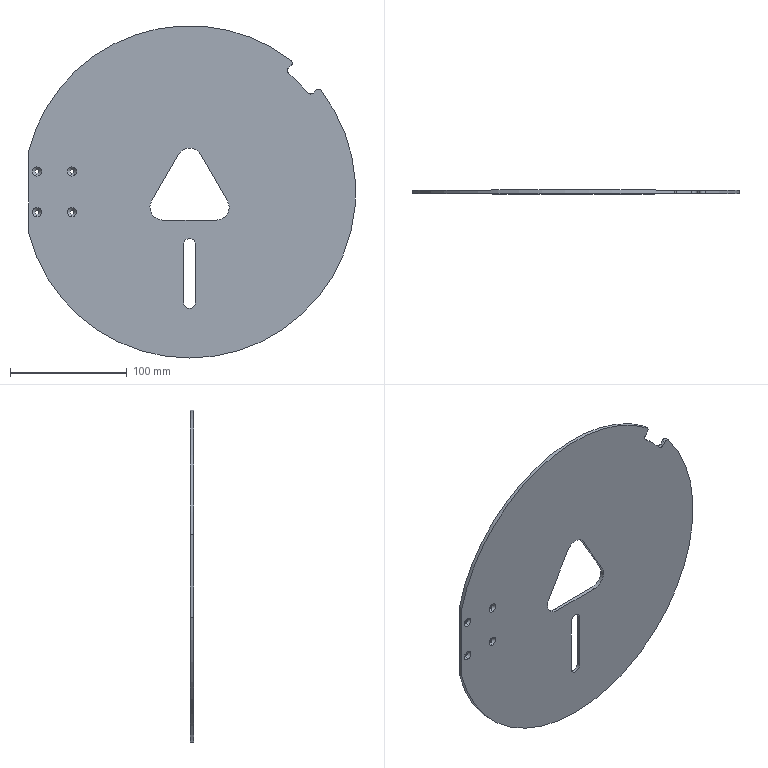Part | SolidWorks | features ICE 5, Chamfer 1, CirPattern 1, Cut 1, Extrusion 1, Fillet 1 | 1 solid | 41 faces | box 280.5 x 3 x 285 mm | volume 179414 mm3 | cylinder 23 | plane 10 | cone 8 | commonest cylinder face diameters 3.5 x8 6 x4 22 x4 10 x3 285 x3 265 x1
STEP:
#1=CARTESIAN_POINT('',(-100.892,2.2,-15.75));
#2=VERTEX_POINT('',#1);
#3=CARTESIAN_POINT('',(-100.892,2.2,-19.25));
#4=VERTEX_POINT('',#3);
#5=CARTESIAN_POINT('',(-100.892,2.2,-17.5));
#6=DIRECTION('',(0.,-1.,0.));
#7=DIRECTION('',(0.,0.,1.));
#8=AXIS2_PLACEMENT_3D('',#5,#6,#7);
#9=CIRCLE('',#8,1.75);
#10=EDGE_CURVE('',#2,#4,#9,.T.);
#11=ORIENTED_EDGE('',*,*,#10,.F.);
#12=CARTESIAN_POINT('',(-100.892,0.,-13.55));
#13=VERTEX_POINT('',#12);
#14=CARTESIAN_POINT('',(-100.892,0.,-13.55));
#15=DIRECTION('',(0.,-0.7071,0.7071));
#16=VECTOR('',#15,1000.);
#17=LINE('',#14,#16);
#18=EDGE_CURVE('',#2,#13,#17,.T.);
#19=ORIENTED_EDGE('',*,*,#18,.T.);
#20=CARTESIAN_POINT('',(-100.892,0.,-21.45));
#21=VERTEX_POINT('',#20);
#22=CARTESIAN_POINT('',(-100.892,0.,-17.5));
#23=DIRECTION('',(0.,1.,0.));
#24=DIRECTION('',(0.,0.,1.));
#25=AXIS2_PLACEMENT_3D('',#22,#23,#24);
#26=CIRCLE('',#25,3.95);
#27=EDGE_CURVE('',#21,#13,#26,.T.);
#28=ORIENTED_EDGE('',*,*,#27,.F.);
#29=CARTESIAN_POINT('',(-100.892,0.,-21.45));
#30=DIRECTION('',(0.,-0.7071,-0.7071));
#31=VECTOR('',#30,1000.);
#32=LINE('',#29,#31);
#33=EDGE_CURVE('',#4,#21,#32,.T.);
#34=ORIENTED_EDGE('',*,*,#33,.F.);
#35=EDGE_LOOP('',(#11,#19,#28,#34));
#36=FACE_OUTER_BOUND('',#35,.T.);
#37=CARTESIAN_POINT('',(-100.892,0.,-17.5));
#38=DIRECTION('',(0.,-1.,0.));
#39=DIRECTION('',(0.,0.,-1.));
#40=AXIS2_PLACEMENT_3D('',#37,#38,#39);
#41=CONICAL_SURFACE('',#40,3.95,0.7854);
#42=ADVANCED_FACE('',(#36),#41,.F.);
#43=CARTESIAN_POINT('',(-130.892,2.2,-15.75));
#44=VERTEX_POINT('',#43);
#45=CARTESIAN_POINT('',(-130.892,2.2,-19.25));
#46=VERTEX_POINT('',#45);
#47=CARTESIAN_POINT('',(-130.892,2.2,-17.5));
#48=DIRECTION('',(0.,-1.,0.));
#49=DIRECTION('',(0.,0.,1.));
#50=AXIS2_PLACEMENT_3D('',#47,#48,#49);
#51=CIRCLE('',#50,1.75);
#52=EDGE_CURVE('',#44,#46,#51,.T.);
#53=ORIENTED_EDGE('',*,*,#52,.F.);
#54=CARTESIAN_POINT('',(-130.892,0.,-13.55));
#55=VERTEX_POINT('',#54);
#56=CARTESIAN_POINT('',(-130.892,0.,-13.55));
#57=DIRECTION('',(0.,-0.7071,0.7071));
#58=VECTOR('',#57,1000.);
#59=LINE('',#56,#58);
#60=EDGE_CURVE('',#44,#55,#59,.T.);
#61=ORIENTED_EDGE('',*,*,#60,.T.);
#62=CARTESIAN_POINT('',(-130.892,0.,-21.45));
#63=VERTEX_POINT('',#62);
#64=CARTESIAN_POINT('',(-130.892,0.,-17.5));
#65=DIRECTION('',(0.,1.,0.));
#66=DIRECTION('',(0.,0.,1.));
#67=AXIS2_PLACEMENT_3D('',#64,#65,#66);
#68=CIRCLE('',#67,3.95);
#69=EDGE_CURVE('',#63,#55,#68,.T.);
#70=ORIENTED_EDGE('',*,*,#69,.F.);
#71=CARTESIAN_POINT('',(-130.892,0.,-21.45));
#72=DIRECTION('',(0.,-0.7071,-0.7071));
#73=VECTOR('',#72,1000.);
#74=LINE('',#71,#73);
#75=EDGE_CURVE('',#46,#63,#74,.T.);
#76=ORIENTED_EDGE('',*,*,#75,.F.);
#77=EDGE_LOOP('',(#53,#61,#70,#76));
#78=FACE_OUTER_BOUND('',#77,.T.);
#79=CARTESIAN_POINT('',(-130.892,0.,-17.5));
#80=DIRECTION('',(0.,-1.,0.));
#81=DIRECTION('',(0.,0.,-1.));
#82=AXIS2_PLACEMENT_3D('',#79,#80,#81);
#83=CONICAL_SURFACE('',#82,3.95,0.7854);
#84=ADVANCED_FACE('',(#78),#83,.F.);
#85=CARTESIAN_POINT('',(-100.892,2.2,19.25));
#86=VERTEX_POINT('',#85);
#87=CARTESIAN_POINT('',(-100.892,2.2,15.75));
#88=VERTEX_POINT('',#87);
#89=CARTESIAN_POINT('',(-100.892,2.2,17.5));
#90=DIRECTION('',(0.,-1.,0.));
#91=DIRECTION('',(0.,0.,1.));
#92=AXIS2_PLACEMENT_3D('',#89,#90,#91);
#93=CIRCLE('',#92,1.75);
#94=EDGE_CURVE('',#86,#88,#93,.T.);
#95=ORIENTED_EDGE('',*,*,#94,.F.);
#96=CARTESIAN_POINT('',(-100.892,0.,21.45));
#97=VERTEX_POINT('',#96);
#98=CARTESIAN_POINT('',(-100.892,0.,21.45));
#99=DIRECTION('',(0.,-0.7071,0.7071));
#100=VECTOR('',#99,1000.);
#101=LINE('',#98,#100);
#102=EDGE_CURVE('',#86,#97,#101,.T.);
#103=ORIENTED_EDGE('',*,*,#102,.T.);
#104=CARTESIAN_POINT('',(-100.892,0.,13.55));
#105=VERTEX_POINT('',#104);
#106=CARTESIAN_POINT('',(-100.892,0.,17.5));
#107=DIRECTION('',(0.,1.,0.));
#108=DIRECTION('',(0.,0.,1.));
#109=AXIS2_PLACEMENT_3D('',#106,#107,#108);
#110=CIRCLE('',#109,3.95);
#111=EDGE_CURVE('',#105,#97,#110,.T.);
#112=ORIENTED_EDGE('',*,*,#111,.F.);
#113=CARTESIAN_POINT('',(-100.892,0.,13.55));
#114=DIRECTION('',(0.,-0.7071,-0.7071));
#115=VECTOR('',#114,1000.);
#116=LINE('',#113,#115);
#117=EDGE_CURVE('',#88,#105,#116,.T.);
#118=ORIENTED_EDGE('',*,*,#117,.F.);
#119=EDGE_LOOP('',(#95,#103,#112,#118));
#120=FACE_OUTER_BOUND('',#119,.T.);
#121=CARTESIAN_POINT('',(-100.892,0.,17.5));
#122=DIRECTION('',(0.,-1.,0.));
#123=DIRECTION('',(0.,0.,-1.));
#124=AXIS2_PLACEMENT_3D('',#121,#122,#123);
#125=CONICAL_SURFACE('',#124,3.95,0.7854);
#126=ADVANCED_FACE('',(#120),#125,.F.);
#127=CARTESIAN_POINT('',(-130.892,2.2,19.25));
#128=VERTEX_POINT('',#127);
#129=CARTESIAN_POINT('',(-130.892,2.2,15.75));
#130=VERTEX_POINT('',#129);
#131=CARTESIAN_POINT('',(-130.892,2.2,17.5));
#132=DIRECTION('',(0.,-1.,0.));
#133=DIRECTION('',(0.,0.,1.));
#134=AXIS2_PLACEMENT_3D('',#131,#132,#133);
#135=CIRCLE('',#134,1.75);
#136=EDGE_CURVE('',#128,#130,#135,.T.);
#137=ORIENTED_EDGE('',*,*,#136,.F.);
#138=CARTESIAN_POINT('',(-130.892,0.,21.45));
#139=VERTEX_POINT('',#138);
#140=CARTESIAN_POINT('',(-130.892,0.,21.45));
#141=DIRECTION('',(0.,-0.7071,0.7071));
#142=VECTOR('',#141,1000.);
#143=LINE('',#140,#142);
#144=EDGE_CURVE('',#128,#139,#143,.T.);
#145=ORIENTED_EDGE('',*,*,#144,.T.);
#146=CARTESIAN_POINT('',(-130.892,0.,13.55));
#147=VERTEX_POINT('',#146);
#148=CARTESIAN_POINT('',(-130.892,0.,17.5));
#149=DIRECTION('',(0.,1.,0.));
#150=DIRECTION('',(0.,0.,1.));
#151=AXIS2_PLACEMENT_3D('',#148,#149,#150);
#152=CIRCLE('',#151,3.95);
#153=EDGE_CURVE('',#147,#139,#152,.T.);
#154=ORIENTED_EDGE('',*,*,#153,.F.);
#155=CARTESIAN_POINT('',(-130.892,0.,13.55));
#156=DIRECTION('',(0.,-0.7071,-0.7071));
#157=VECTOR('',#156,1000.);
#158=LINE('',#155,#157);
#159=EDGE_CURVE('',#130,#147,#158,.T.);
#160=ORIENTED_EDGE('',*,*,#159,.F.);
#161=EDGE_LOOP('',(#137,#145,#154,#160));
#162=FACE_OUTER_BOUND('',#161,.T.);
#163=CARTESIAN_POINT('',(-130.892,0.,17.5));
#164=DIRECTION('',(0.,-1.,0.));
#165=DIRECTION('',(0.,0.,-1.));
#166=AXIS2_PLACEMENT_3D('',#163,#164,#165);
#167=CONICAL_SURFACE('',#166,3.95,0.7854);
#168=ADVANCED_FACE('',(#162),#167,.F.);
#169=ORIENTED_EDGE('',*,*,#94,.T.);
#170=CARTESIAN_POINT('',(-100.892,3.,15.75));
#171=VERTEX_POINT('',#170);
#172=CARTESIAN_POINT('',(-100.892,-7.,15.75));
#173=DIRECTION('',(0.,1.,0.));
#174=VECTOR('',#173,1000.);
#175=LINE('',#172,#174);
#176=EDGE_CURVE('',#88,#171,#175,.T.);
#177=ORIENTED_EDGE('',*,*,#176,.T.);
#178=CARTESIAN_POINT('',(-100.892,3.,19.25));
#179=VERTEX_POINT('',#178);
#180=CARTESIAN_POINT('',(-100.892,3.,17.5));
#181=DIRECTION('',(0.,1.,0.));
#182=DIRECTION('',(0.,0.,1.));
#183=AXIS2_PLACEMENT_3D('',#180,#181,#182);
#184=CIRCLE('',#183,1.75);
#185=EDGE_CURVE('',#171,#179,#184,.T.);
#186=ORIENTED_EDGE('',*,*,#185,.T.);
#187=CARTESIAN_POINT('',(-100.892,-7.,19.25));
#188=DIRECTION('',(0.,1.,0.));
#189=VECTOR('',#188,1000.);
#190=LINE('',#187,#189);
#191=EDGE_CURVE('',#86,#179,#190,.T.);
#192=ORIENTED_EDGE('',*,*,#191,.F.);
#193=EDGE_LOOP('',(#169,#177,#186,#192));
#194=FACE_OUTER_BOUND('',#193,.T.);
#195=CARTESIAN_POINT('',(-100.892,-7.,17.5));
#196=DIRECTION('',(0.,1.,0.));
#197=DIRECTION('',(0.,0.,1.));
#198=AXIS2_PLACEMENT_3D('',#195,#196,#197);
#199=CYLINDRICAL_SURFACE('',#198,1.75);
#200=ADVANCED_FACE('',(#194),#199,.F.);
#201=ORIENTED_EDGE('',*,*,#136,.T.);
#202=CARTESIAN_POINT('',(-130.892,3.,15.75));
#203=VERTEX_POINT('',#202);
#204=CARTESIAN_POINT('',(-130.892,-7.,15.75));
#205=DIRECTION('',(0.,1.,0.));
#206=VECTOR('',#205,1000.);
#207=LINE('',#204,#206);
#208=EDGE_CURVE('',#130,#203,#207,.T.);
#209=ORIENTED_EDGE('',*,*,#208,.T.);
#210=CARTESIAN_POINT('',(-130.892,3.,19.25));
#211=VERTEX_POINT('',#210);
#212=CARTESIAN_POINT('',(-130.892,3.,17.5));
#213=DIRECTION('',(0.,1.,0.));
#214=DIRECTION('',(0.,0.,1.));
#215=AXIS2_PLACEMENT_3D('',#212,#213,#214);
#216=CIRCLE('',#215,1.75);
#217=EDGE_CURVE('',#203,#211,#216,.T.);
#218=ORIENTED_EDGE('',*,*,#217,.T.);
#219=CARTESIAN_POINT('',(-130.892,-7.,19.25));
#220=DIRECTION('',(0.,1.,0.));
#221=VECTOR('',#220,1000.);
#222=LINE('',#219,#221);
#223=EDGE_CURVE('',#128,#211,#222,.T.);
#224=ORIENTED_EDGE('',*,*,#223,.F.);
#225=EDGE_LOOP('',(#201,#209,#218,#224));
#226=FACE_OUTER_BOUND('',#225,.T.);
#227=CARTESIAN_POINT('',(-130.892,-7.,17.5));
#228=DIRECTION('',(0.,1.,0.));
#229=DIRECTION('',(0.,0.,1.));
#230=AXIS2_PLACEMENT_3D('',#227,#228,#229);
#231=CYLINDRICAL_SURFACE('',#230,1.75);
#232=ADVANCED_FACE('',(#226),#231,.F.);
#233=ORIENTED_EDGE('',*,*,#10,.T.);
#234=CARTESIAN_POINT('',(-100.892,3.,-19.25));
#235=VERTEX_POINT('',#234);
#236=CARTESIAN_POINT('',(-100.892,-7.,-19.25));
#237=DIRECTION('',(0.,1.,0.));
#238=VECTOR('',#237,1000.);
#239=LINE('',#236,#238);
#240=EDGE_CURVE('',#4,#235,#239,.T.);
#241=ORIENTED_EDGE('',*,*,#240,.T.);
#242=CARTESIAN_POINT('',(-100.892,3.,-15.75));
#243=VERTEX_POINT('',#242);
#244=CARTESIAN_POINT('',(-100.892,3.,-17.5));
#245=DIRECTION('',(0.,1.,0.));
#246=DIRECTION('',(0.,0.,1.));
#247=AXIS2_PLACEMENT_3D('',#244,#245,#246);
#248=CIRCLE('',#247,1.75);
#249=EDGE_CURVE('',#235,#243,#248,.T.);
#250=ORIENTED_EDGE('',*,*,#249,.T.);
#251=CARTESIAN_POINT('',(-100.892,-7.,-15.75));
#252=DIRECTION('',(0.,1.,0.));
#253=VECTOR('',#252,1000.);
#254=LINE('',#251,#253);
#255=EDGE_CURVE('',#2,#243,#254,.T.);
#256=ORIENTED_EDGE('',*,*,#255,.F.);
#257=EDGE_LOOP('',(#233,#241,#250,#256));
#258=FACE_OUTER_BOUND('',#257,.T.);
#259=CARTESIAN_POINT('',(-100.892,-7.,-17.5));
#260=DIRECTION('',(0.,1.,0.));
#261=DIRECTION('',(0.,0.,1.));
#262=AXIS2_PLACEMENT_3D('',#259,#260,#261);
#263=CYLINDRICAL_SURFACE('',#262,1.75);
#264=ADVANCED_FACE('',(#258),#263,.F.);
#265=ORIENTED_EDGE('',*,*,#52,.T.);
#266=CARTESIAN_POINT('',(-130.892,3.,-19.25));
#267=VERTEX_POINT('',#266);
#268=CARTESIAN_POINT('',(-130.892,-7.,-19.25));
#269=DIRECTION('',(0.,1.,0.));
#270=VECTOR('',#269,1000.);
#271=LINE('',#268,#270);
#272=EDGE_CURVE('',#46,#267,#271,.T.);
#273=ORIENTED_EDGE('',*,*,#272,.T.);
#274=CARTESIAN_POINT('',(-130.892,3.,-15.75));
#275=VERTEX_POINT('',#274);
#276=CARTESIAN_POINT('',(-130.892,3.,-17.5));
#277=DIRECTION('',(0.,1.,0.));
#278=DIRECTION('',(0.,0.,1.));
#279=AXIS2_PLACEMENT_3D('',#276,#277,#278);
#280=CIRCLE('',#279,1.75);
#281=EDGE_CURVE('',#267,#275,#280,.T.);
#282=ORIENTED_EDGE('',*,*,#281,.T.);
#283=CARTESIAN_POINT('',(-130.892,-7.,-15.75));
#284=DIRECTION('',(0.,1.,0.));
#285=VECTOR('',#284,1000.);
#286=LINE('',#283,#285);
#287=EDGE_CURVE('',#44,#275,#286,.T.);
#288=ORIENTED_EDGE('',*,*,#287,.F.);
#289=EDGE_LOOP('',(#265,#273,#282,#288));
#290=FACE_OUTER_BOUND('',#289,.T.);
#291=CARTESIAN_POINT('',(-130.892,-7.,-17.5));
#292=DIRECTION('',(0.,1.,0.));
#293=DIRECTION('',(0.,0.,1.));
#294=AXIS2_PLACEMENT_3D('',#291,#292,#293);
#295=CYLINDRICAL_SURFACE('',#294,1.75);
#296=ADVANCED_FACE('',(#290),#295,.F.);
#297=CARTESIAN_POINT('',(0.,0.,-40.));
#298=VERTEX_POINT('',#297);
#299=CARTESIAN_POINT('',(5.,0.,-45.));
#300=VERTEX_POINT('',#299);
#301=CARTESIAN_POINT('',(0.,0.,-45.));
#302=DIRECTION('',(0.,1.,0.));
#303=DIRECTION('',(0.,0.,1.));
#304=AXIS2_PLACEMENT_3D('',#301,#302,#303);
#305=CIRCLE('',#304,5.);
#306=EDGE_CURVE('',#298,#300,#305,.T.);
#307=ORIENTED_EDGE('',*,*,#306,.F.);
#308=CARTESIAN_POINT('',(0.,3.,-40.));
#309=VERTEX_POINT('',#308);
#310=CARTESIAN_POINT('',(0.,-7.,-40.));
#311=DIRECTION('',(0.,1.,0.));
#312=VECTOR('',#311,1000.);
#313=LINE('',#310,#312);
#314=EDGE_CURVE('',#298,#309,#313,.T.);
#315=ORIENTED_EDGE('',*,*,#314,.T.);
#316=CARTESIAN_POINT('',(5.,3.,-45.));
#317=VERTEX_POINT('',#316);
#318=CARTESIAN_POINT('',(0.,3.,-45.));
#319=DIRECTION('',(0.,1.,0.));
#320=DIRECTION('',(0.,0.,1.));
#321=AXIS2_PLACEMENT_3D('',#318,#319,#320);
#322=CIRCLE('',#321,5.);
#323=EDGE_CURVE('',#309,#317,#322,.T.);
#324=ORIENTED_EDGE('',*,*,#323,.T.);
#325=CARTESIAN_POINT('',(5.,-7.,-45.));
#326=DIRECTION('',(0.,1.,0.));
#327=VECTOR('',#326,1000.);
#328=LINE('',#325,#327);
#329=EDGE_CURVE('',#300,#317,#328,.T.);
#330=ORIENTED_EDGE('',*,*,#329,.F.);
#331=EDGE_LOOP('',(#307,#315,#324,#330));
#332=FACE_OUTER_BOUND('',#331,.T.);
#333=CARTESIAN_POINT('',(0.,-7.,-45.));
#334=DIRECTION('',(0.,1.,0.));
#335=DIRECTION('',(0.,0.,1.));
#336=AXIS2_PLACEMENT_3D('',#333,#334,#335);
#337=CYLINDRICAL_SURFACE('',#336,5.);
#338=ADVANCED_FACE('',(#332),#337,.F.);
#339=CARTESIAN_POINT('',(0.,3.,-142.5));
#340=VERTEX_POINT('',#339);
#341=CARTESIAN_POINT('',(-138.,3.,-35.528));
#342=VERTEX_POINT('',#341);
#343=CARTESIAN_POINT('',(0.,3.,0.));
#344=DIRECTION('',(0.,1.,0.));
#345=DIRECTION('',(0.,0.,1.));
#346=AXIS2_PLACEMENT_3D('',#343,#344,#345);
#347=CIRCLE('',#346,142.5);
#348=EDGE_CURVE('',#340,#342,#347,.T.);
#349=ORIENTED_EDGE('',*,*,#348,.F.);
#350=CARTESIAN_POINT('',(0.,0.,-142.5));
#351=VERTEX_POINT('',#350);
#352=CARTESIAN_POINT('',(0.,3.,-142.5));
#353=DIRECTION('',(0.,-1.,0.));
#354=VECTOR('',#353,1000.);
#355=LINE('',#352,#354);
#356=EDGE_CURVE('',#340,#351,#355,.T.);
#357=ORIENTED_EDGE('',*,*,#356,.T.);
#358=CARTESIAN_POINT('',(-138.,0.,-35.528));
#359=VERTEX_POINT('',#358);
#360=CARTESIAN_POINT('',(0.,0.,0.));
#361=DIRECTION('',(0.,1.,0.));
#362=DIRECTION('',(0.,0.,1.));
#363=AXIS2_PLACEMENT_3D('',#360,#361,#362);
#364=CIRCLE('',#363,142.5);
#365=EDGE_CURVE('',#351,#359,#364,.T.);
#366=ORIENTED_EDGE('',*,*,#365,.T.);
#367=CARTESIAN_POINT('',(-138.,3.,-35.528));
#368=DIRECTION('',(0.,1.,0.));
#369=VECTOR('',#368,1000.);
#370=LINE('',#367,#369);
#371=EDGE_CURVE('',#359,#342,#370,.T.);
#372=ORIENTED_EDGE('',*,*,#371,.T.);
#373=EDGE_LOOP('',(#349,#357,#366,#372));
#374=FACE_OUTER_BOUND('',#373,.T.);
#375=CARTESIAN_POINT('',(0.,3.,0.));
#376=DIRECTION('',(0.,-1.,0.));
#377=DIRECTION('',(0.,0.,-1.));
#378=AXIS2_PLACEMENT_3D('',#375,#376,#377);
#379=CYLINDRICAL_SURFACE('',#378,142.5);
#380=ADVANCED_FACE('',(#374),#379,.T.);
#381=CARTESIAN_POINT('',(0.,0.,37.5));
#382=VERTEX_POINT('',#381);
#383=CARTESIAN_POINT('',(9.526,0.,32.));
#384=VERTEX_POINT('',#383);
#385=CARTESIAN_POINT('',(0.,0.,26.5));
#386=DIRECTION('',(0.,1.,0.));
#387=DIRECTION('',(0.,0.,1.));
#388=AXIS2_PLACEMENT_3D('',#385,#386,#387);
#389=CIRCLE('',#388,11.);
#390=EDGE_CURVE('',#382,#384,#389,.T.);
#391=ORIENTED_EDGE('',*,*,#390,.F.);
#392=CARTESIAN_POINT('',(0.,3.,37.5));
#393=VERTEX_POINT('',#392);
#394=CARTESIAN_POINT('',(0.,-7.,37.5));
#395=DIRECTION('',(0.,1.,0.));
#396=VECTOR('',#395,1000.);
#397=LINE('',#394,#396);
#398=EDGE_CURVE('',#382,#393,#397,.T.);
#399=ORIENTED_EDGE('',*,*,#398,.T.);
#400=CARTESIAN_POINT('',(9.526,3.,32.));
#401=VERTEX_POINT('',#400);
#402=CARTESIAN_POINT('',(0.,3.,26.5));
#403=DIRECTION('',(0.,1.,0.));
#404=DIRECTION('',(0.,0.,1.));
#405=AXIS2_PLACEMENT_3D('',#402,#403,#404);
#406=CIRCLE('',#405,11.);
#407=EDGE_CURVE('',#393,#401,#406,.T.);
#408=ORIENTED_EDGE('',*,*,#407,.T.);
#409=CARTESIAN_POINT('',(9.526,-7.,32.));
#410=DIRECTION('',(0.,1.,0.));
#411=VECTOR('',#410,1000.);
#412=LINE('',#409,#411);
#413=EDGE_CURVE('',#384,#401,#412,.T.);
#414=ORIENTED_EDGE('',*,*,#413,.F.);
#415=EDGE_LOOP('',(#391,#399,#408,#414));
#416=FACE_OUTER_BOUND('',#415,.T.);
#417=CARTESIAN_POINT('',(0.,-7.,26.5));
#418=DIRECTION('',(0.,1.,0.));
#419=DIRECTION('',(0.,0.,1.));
#420=AXIS2_PLACEMENT_3D('',#417,#418,#419);
#421=CYLINDRICAL_SURFACE('',#420,11.);
#422=ADVANCED_FACE('',(#416),#421,.F.);
#423=CARTESIAN_POINT('',(-138.,3.,35.528));
#424=VERTEX_POINT('',#423);
#425=CARTESIAN_POINT('',(86.919,3.,112.922));
#426=VERTEX_POINT('',#425);
#427=CARTESIAN_POINT('',(0.,3.,0.));
#428=DIRECTION('',(0.,1.,0.));
#429=DIRECTION('',(0.,0.,1.));
#430=AXIS2_PLACEMENT_3D('',#427,#428,#429);
#431=CIRCLE('',#430,142.5);
#432=EDGE_CURVE('',#424,#426,#431,.T.);
#433=ORIENTED_EDGE('',*,*,#432,.F.);
#434=CARTESIAN_POINT('',(-138.,0.,35.528));
#435=VERTEX_POINT('',#434);
#436=CARTESIAN_POINT('',(-138.,3.,35.528));
#437=DIRECTION('',(0.,-1.,0.));
#438=VECTOR('',#437,1000.);
#439=LINE('',#436,#438);
#440=EDGE_CURVE('',#424,#435,#439,.T.);
#441=ORIENTED_EDGE('',*,*,#440,.T.);
#442=CARTESIAN_POINT('',(86.919,0.,112.922));
#443=VERTEX_POINT('',#442);
#444=CARTESIAN_POINT('',(0.,0.,0.));
#445=DIRECTION('',(0.,1.,0.));
#446=DIRECTION('',(0.,0.,1.));
#447=AXIS2_PLACEMENT_3D('',#444,#445,#446);
#448=CIRCLE('',#447,142.5);
#449=EDGE_CURVE('',#435,#443,#448,.T.);
#450=ORIENTED_EDGE('',*,*,#449,.T.);
#451=CARTESIAN_POINT('',(86.919,3.,112.922));
#452=DIRECTION('',(0.,1.,0.));
#453=VECTOR('',#452,1000.);
#454=LINE('',#451,#453);
#455=EDGE_CURVE('',#443,#426,#454,.T.);
#456=ORIENTED_EDGE('',*,*,#455,.T.);
#457=EDGE_LOOP('',(#433,#441,#450,#456));
#458=FACE_OUTER_BOUND('',#457,.T.);
#459=CARTESIAN_POINT('',(0.,3.,0.));
#460=DIRECTION('',(0.,-1.,0.));
#461=DIRECTION('',(0.,0.,-1.));
#462=AXIS2_PLACEMENT_3D('',#459,#460,#461);
#463=CYLINDRICAL_SURFACE('',#462,142.5);
#464=ADVANCED_FACE('',(#458),#463,.T.);
#465=ORIENTED_EDGE('',*,*,#398,.F.);
#466=CARTESIAN_POINT('',(-9.526,0.,32.));
#467=VERTEX_POINT('',#466);
#468=CARTESIAN_POINT('',(0.,0.,26.5));
#469=DIRECTION('',(0.,1.,0.));
#470=DIRECTION('',(0.,0.,1.));
#471=AXIS2_PLACEMENT_3D('',#468,#469,#470);
#472=CIRCLE('',#471,11.);
#473=EDGE_CURVE('',#467,#382,#472,.T.);
#474=ORIENTED_EDGE('',*,*,#473,.F.);
#475=CARTESIAN_POINT('',(-9.526,3.,32.));
#476=VERTEX_POINT('',#475);
#477=CARTESIAN_POINT('',(-9.526,-7.,32.));
#478=DIRECTION('',(0.,1.,0.));
#479=VECTOR('',#478,1000.);
#480=LINE('',#477,#479);
#481=EDGE_CURVE('',#467,#476,#480,.T.);
#482=ORIENTED_EDGE('',*,*,#481,.T.);
#483=CARTESIAN_POINT('',(0.,3.,26.5));
#484=DIRECTION('',(0.,1.,0.));
#485=DIRECTION('',(0.,0.,1.));
#486=AXIS2_PLACEMENT_3D('',#483,#484,#485);
#487=CIRCLE('',#486,11.);
#488=EDGE_CURVE('',#476,#393,#487,.T.);
#489=ORIENTED_EDGE('',*,*,#488,.T.);
#490=EDGE_LOOP('',(#465,#474,#482,#489));
#491=FACE_OUTER_BOUND('',#490,.T.);
#492=CARTESIAN_POINT('',(0.,-7.,26.5));
#493=DIRECTION('',(0.,1.,0.));
#494=DIRECTION('',(0.,0.,1.));
#495=AXIS2_PLACEMENT_3D('',#492,#493,#494);
#496=CYLINDRICAL_SURFACE('',#495,11.);
#497=ADVANCED_FACE('',(#491),#496,.F.);
#498=ORIENTED_EDGE('',*,*,#356,.F.);
#499=CARTESIAN_POINT('',(112.922,3.,86.919));
#500=VERTEX_POINT('',#499);
#501=CARTESIAN_POINT('',(0.,3.,0.));
#502=DIRECTION('',(0.,1.,0.));
#503=DIRECTION('',(0.,0.,1.));
#504=AXIS2_PLACEMENT_3D('',#501,#502,#503);
#505=CIRCLE('',#504,142.5);
#506=EDGE_CURVE('',#500,#340,#505,.T.);
#507=ORIENTED_EDGE('',*,*,#506,.F.);
#508=CARTESIAN_POINT('',(112.922,0.,86.919));
#509=VERTEX_POINT('',#508);
#510=CARTESIAN_POINT('',(112.922,3.,86.919));
#511=DIRECTION('',(0.,-1.,0.));
#512=VECTOR('',#511,1000.);
#513=LINE('',#510,#512);
#514=EDGE_CURVE('',#500,#509,#513,.T.);
#515=ORIENTED_EDGE('',*,*,#514,.T.);
#516=CARTESIAN_POINT('',(0.,0.,0.));
#517=DIRECTION('',(0.,1.,0.));
#518=DIRECTION('',(0.,0.,1.));
#519=AXIS2_PLACEMENT_3D('',#516,#517,#518);
#520=CIRCLE('',#519,142.5);
#521=EDGE_CURVE('',#509,#351,#520,.T.);
#522=ORIENTED_EDGE('',*,*,#521,.T.);
#523=EDGE_LOOP('',(#498,#507,#515,#522));
#524=FACE_OUTER_BOUND('',#523,.T.);
#525=CARTESIAN_POINT('',(0.,3.,0.));
#526=DIRECTION('',(0.,-1.,0.));
#527=DIRECTION('',(0.,0.,-1.));
#528=AXIS2_PLACEMENT_3D('',#525,#526,#527);
#529=CYLINDRICAL_SURFACE('',#528,142.5);
#530=ADVANCED_FACE('',(#524),#529,.T.);
#531=CARTESIAN_POINT('',(-100.892,3.,17.5));
#532=DIRECTION('',(0.,1.,0.));
#533=DIRECTION('',(0.,0.,1.));
#534=AXIS2_PLACEMENT_3D('',#531,#532,#533);
#535=CIRCLE('',#534,1.75);
#536=EDGE_CURVE('',#179,#171,#535,.T.);
#537=ORIENTED_EDGE('',*,*,#536,.F.);
#538=ORIENTED_EDGE('',*,*,#185,.F.);
#539=EDGE_LOOP('',(#537,#538));
#540=FACE_BOUND('',#539,.T.);
#541=CARTESIAN_POINT('',(-130.892,3.,17.5));
#542=DIRECTION('',(0.,1.,0.));
#543=DIRECTION('',(0.,0.,1.));
#544=AXIS2_PLACEMENT_3D('',#541,#542,#543);
#545=CIRCLE('',#544,1.75);
#546=EDGE_CURVE('',#211,#203,#545,.T.);
#547=ORIENTED_EDGE('',*,*,#546,.F.);
#548=ORIENTED_EDGE('',*,*,#217,.F.);
#549=EDGE_LOOP('',(#547,#548));
#550=FACE_BOUND('',#549,.T.);
#551=CARTESIAN_POINT('',(-100.892,3.,-17.5));
#552=DIRECTION('',(0.,1.,0.));
#553=DIRECTION('',(0.,0.,1.));
#554=AXIS2_PLACEMENT_3D('',#551,#552,#553);
#555=CIRCLE('',#554,1.75);
#556=EDGE_CURVE('',#243,#235,#555,.T.);
#557=ORIENTED_EDGE('',*,*,#556,.F.);
#558=ORIENTED_EDGE('',*,*,#249,.F.);
#559=EDGE_LOOP('',(#557,#558));
#560=FACE_BOUND('',#559,.T.);
#561=CARTESIAN_POINT('',(-130.892,3.,-17.5));
#562=DIRECTION('',(0.,1.,0.));
#563=DIRECTION('',(0.,0.,1.));
#564=AXIS2_PLACEMENT_3D('',#561,#562,#563);
#565=CIRCLE('',#564,1.75);
#566=EDGE_CURVE('',#275,#267,#565,.T.);
#567=ORIENTED_EDGE('',*,*,#566,.F.);
#568=ORIENTED_EDGE('',*,*,#281,.F.);
#569=EDGE_LOOP('',(#567,#568));
#570=FACE_BOUND('',#569,.T.);
#571=CARTESIAN_POINT('',(-138.,3.,-60.));
#572=DIRECTION('',(0.,0.,-1.));
#573=VECTOR('',#572,1000.);
#574=LINE('',#571,#573);
#575=EDGE_CURVE('',#424,#342,#574,.T.);
#576=ORIENTED_EDGE('',*,*,#575,.F.);
#577=ORIENTED_EDGE('',*,*,#432,.T.);
#578=CARTESIAN_POINT('',(87.21,3.,108.423));
#579=VERTEX_POINT('',#578);
#580=CARTESIAN_POINT('',(85.089,3.,110.545));
#581=DIRECTION('',(0.,1.,0.));
#582=DIRECTION('',(0.,0.,1.));
#583=AXIS2_PLACEMENT_3D('',#580,#581,#582);
#584=CIRCLE('',#583,3.);
#585=EDGE_CURVE('',#426,#579,#584,.T.);
#586=ORIENTED_EDGE('',*,*,#585,.T.);
#587=CARTESIAN_POINT('',(84.83,3.,106.043));
#588=VERTEX_POINT('',#587);
#589=CARTESIAN_POINT('',(89.596,3.,110.81));
#590=DIRECTION('',(0.7071,0.,0.7071));
#591=VECTOR('',#590,1000.);
#592=LINE('',#589,#591);
#593=EDGE_CURVE('',#588,#579,#592,.T.);
#594=ORIENTED_EDGE('',*,*,#593,.F.);
#595=CARTESIAN_POINT('',(85.026,3.,101.621));
#596=VERTEX_POINT('',#595);
#597=CARTESIAN_POINT('',(86.951,3.,103.922));
#598=DIRECTION('',(0.,-1.,0.));
#599=DIRECTION('',(0.,0.,1.));
#600=AXIS2_PLACEMENT_3D('',#597,#598,#599);
#601=CIRCLE('',#600,3.);
#602=EDGE_CURVE('',#588,#596,#601,.T.);
#603=ORIENTED_EDGE('',*,*,#602,.T.);
#604=CARTESIAN_POINT('',(101.621,3.,85.026));
#605=VERTEX_POINT('',#604);
#606=CARTESIAN_POINT('',(0.,3.,0.));
#607=DIRECTION('',(0.,-1.,0.));
#608=DIRECTION('',(0.,0.,1.));
#609=AXIS2_PLACEMENT_3D('',#606,#607,#608);
#610=CIRCLE('',#609,132.5);
#611=EDGE_CURVE('',#605,#596,#610,.T.);
#612=ORIENTED_EDGE('',*,*,#611,.F.);
#613=CARTESIAN_POINT('',(106.043,3.,84.83));
#614=VERTEX_POINT('',#613);
#615=CARTESIAN_POINT('',(103.922,3.,86.951));
#616=DIRECTION('',(0.,-1.,0.));
#617=DIRECTION('',(0.,0.,1.));
#618=AXIS2_PLACEMENT_3D('',#615,#616,#617);
#619=CIRCLE('',#618,3.);
#620=EDGE_CURVE('',#605,#614,#619,.T.);
#621=ORIENTED_EDGE('',*,*,#620,.T.);
#622=CARTESIAN_POINT('',(108.423,3.,87.21));
#623=VERTEX_POINT('',#622);
#624=CARTESIAN_POINT('',(110.81,3.,89.596));
#625=DIRECTION('',(-0.7071,0.,-0.7071));
#626=VECTOR('',#625,1000.);
#627=LINE('',#624,#626);
#628=EDGE_CURVE('',#623,#614,#627,.T.);
#629=ORIENTED_EDGE('',*,*,#628,.F.);
#630=CARTESIAN_POINT('',(110.545,3.,85.089));
#631=DIRECTION('',(0.,1.,0.));
#632=DIRECTION('',(0.,0.,1.));
#633=AXIS2_PLACEMENT_3D('',#630,#631,#632);
#634=CIRCLE('',#633,3.);
#635=EDGE_CURVE('',#623,#500,#634,.T.);
#636=ORIENTED_EDGE('',*,*,#635,.T.);
#637=ORIENTED_EDGE('',*,*,#506,.T.);
#638=ORIENTED_EDGE('',*,*,#348,.T.);
#639=EDGE_LOOP('',(#576,#577,#586,#594,#603,#612,#621,#629,#636,#637,#638));
#640=FACE_OUTER_BOUND('',#639,.T.);
#641=CARTESIAN_POINT('',(-5.,3.,-45.));
#642=VERTEX_POINT('',#641);
#643=CARTESIAN_POINT('',(0.,3.,-45.));
#644=DIRECTION('',(0.,1.,0.));
#645=DIRECTION('',(0.,0.,1.));
#646=AXIS2_PLACEMENT_3D('',#643,#644,#645);
#647=CIRCLE('',#646,5.);
#648=EDGE_CURVE('',#642,#309,#647,.T.);
#649=ORIENTED_EDGE('',*,*,#648,.F.);
#650=CARTESIAN_POINT('',(-5.,3.,-95.));
#651=VERTEX_POINT('',#650);
#652=CARTESIAN_POINT('',(-5.,3.,-45.));
#653=DIRECTION('',(0.,0.,1.));
#654=VECTOR('',#653,1000.);
#655=LINE('',#652,#654);
#656=EDGE_CURVE('',#651,#642,#655,.T.);
#657=ORIENTED_EDGE('',*,*,#656,.F.);
#658=CARTESIAN_POINT('',(5.,3.,-95.));
#659=VERTEX_POINT('',#658);
#660=CARTESIAN_POINT('',(0.,3.,-95.));
#661=DIRECTION('',(0.,1.,0.));
#662=DIRECTION('',(0.,0.,1.));
#663=AXIS2_PLACEMENT_3D('',#660,#661,#662);
#664=CIRCLE('',#663,5.);
#665=EDGE_CURVE('',#659,#651,#664,.T.);
#666=ORIENTED_EDGE('',*,*,#665,.F.);
#667=CARTESIAN_POINT('',(5.,3.,-45.));
#668=DIRECTION('',(0.,0.,-1.));
#669=VECTOR('',#668,1000.);
#670=LINE('',#667,#669);
#671=EDGE_CURVE('',#317,#659,#670,.T.);
#672=ORIENTED_EDGE('',*,*,#671,.F.);
#673=ORIENTED_EDGE('',*,*,#323,.F.);
#674=EDGE_LOOP('',(#649,#657,#666,#672,#673));
#675=FACE_BOUND('',#674,.T.);
#676=CARTESIAN_POINT('',(-32.476,3.,-7.75));
#677=VERTEX_POINT('',#676);
#678=CARTESIAN_POINT('',(-32.476,3.,-7.75));
#679=DIRECTION('',(0.5,0.,0.866));
#680=VECTOR('',#679,1000.);
#681=LINE('',#678,#680);
#682=EDGE_CURVE('',#677,#476,#681,.T.);
#683=ORIENTED_EDGE('',*,*,#682,.F.);
#684=CARTESIAN_POINT('',(-22.95,3.,-24.25));
#685=VERTEX_POINT('',#684);
#686=CARTESIAN_POINT('',(-22.95,3.,-13.25));
#687=DIRECTION('',(0.,1.,0.));
#688=DIRECTION('',(-0.866,0.,-0.5));
#689=AXIS2_PLACEMENT_3D('',#686,#687,#688);
#690=CIRCLE('',#689,11.);
#691=EDGE_CURVE('',#685,#677,#690,.T.);
#692=ORIENTED_EDGE('',*,*,#691,.F.);
#693=CARTESIAN_POINT('',(22.95,3.,-24.25));
#694=VERTEX_POINT('',#693);
#695=CARTESIAN_POINT('',(-22.95,3.,-24.25));
#696=DIRECTION('',(-1.,0.,0.));
#697=VECTOR('',#696,1000.);
#698=LINE('',#695,#697);
#699=EDGE_CURVE('',#694,#685,#698,.T.);
#700=ORIENTED_EDGE('',*,*,#699,.F.);
#701=CARTESIAN_POINT('',(32.476,3.,-7.75));
#702=VERTEX_POINT('',#701);
#703=CARTESIAN_POINT('',(22.95,3.,-13.25));
#704=DIRECTION('',(0.,1.,0.));
#705=DIRECTION('',(0.866,0.,-0.5));
#706=AXIS2_PLACEMENT_3D('',#703,#704,#705);
#707=CIRCLE('',#706,11.);
#708=EDGE_CURVE('',#702,#694,#707,.T.);
#709=ORIENTED_EDGE('',*,*,#708,.F.);
#710=CARTESIAN_POINT('',(32.476,3.,-7.75));
#711=DIRECTION('',(0.5,0.,-0.866));
#712=VECTOR('',#711,1000.);
#713=LINE('',#710,#712);
#714=EDGE_CURVE('',#401,#702,#713,.T.);
#715=ORIENTED_EDGE('',*,*,#714,.F.);
#716=ORIENTED_EDGE('',*,*,#407,.F.);
#717=ORIENTED_EDGE('',*,*,#488,.F.);
#718=EDGE_LOOP('',(#683,#692,#700,#709,#715,#716,#717));
#719=FACE_BOUND('',#718,.T.);
#720=CARTESIAN_POINT('',(0.,3.,0.));
#721=DIRECTION('',(0.,1.,0.));
#722=DIRECTION('',(0.,0.,1.));
#723=AXIS2_PLACEMENT_3D('',#720,#721,#722);
#724=PLANE('',#723);
#725=ADVANCED_FACE('',(#540,#550,#560,#570,#640,#675,#719),#724,.T.);
#726=ORIENTED_EDGE('',*,*,#153,.T.);
#727=CARTESIAN_POINT('',(-130.892,0.,17.5));
#728=DIRECTION('',(0.,1.,0.));
#729=DIRECTION('',(0.,0.,1.));
#730=AXIS2_PLACEMENT_3D('',#727,#728,#729);
#731=CIRCLE('',#730,3.95);
#732=EDGE_CURVE('',#139,#147,#731,.T.);
#733=ORIENTED_EDGE('',*,*,#732,.T.);
#734=EDGE_LOOP('',(#726,#733));
#735=FACE_BOUND('',#734,.T.);
#736=ORIENTED_EDGE('',*,*,#111,.T.);
#737=CARTESIAN_POINT('',(-100.892,0.,17.5));
#738=DIRECTION('',(0.,1.,0.));
#739=DIRECTION('',(0.,0.,1.));
#740=AXIS2_PLACEMENT_3D('',#737,#738,#739);
#741=CIRCLE('',#740,3.95);
#742=EDGE_CURVE('',#97,#105,#741,.T.);
#743=ORIENTED_EDGE('',*,*,#742,.T.);
#744=EDGE_LOOP('',(#736,#743));
#745=FACE_BOUND('',#744,.T.);
#746=ORIENTED_EDGE('',*,*,#69,.T.);
#747=CARTESIAN_POINT('',(-130.892,0.,-17.5));
#748=DIRECTION('',(0.,1.,0.));
#749=DIRECTION('',(0.,0.,1.));
#750=AXIS2_PLACEMENT_3D('',#747,#748,#749);
#751=CIRCLE('',#750,3.95);
#752=EDGE_CURVE('',#55,#63,#751,.T.);
#753=ORIENTED_EDGE('',*,*,#752,.T.);
#754=EDGE_LOOP('',(#746,#753));
#755=FACE_BOUND('',#754,.T.);
#756=ORIENTED_EDGE('',*,*,#27,.T.);
#757=CARTESIAN_POINT('',(-100.892,0.,-17.5));
#758=DIRECTION('',(0.,1.,0.));
#759=DIRECTION('',(0.,0.,1.));
#760=AXIS2_PLACEMENT_3D('',#757,#758,#759);
#761=CIRCLE('',#760,3.95);
#762=EDGE_CURVE('',#13,#21,#761,.T.);
#763=ORIENTED_EDGE('',*,*,#762,.T.);
#764=EDGE_LOOP('',(#756,#763));
#765=FACE_BOUND('',#764,.T.);
#766=CARTESIAN_POINT('',(-5.,0.,-95.));
#767=VERTEX_POINT('',#766);
#768=CARTESIAN_POINT('',(-5.,0.,-45.));
#769=VERTEX_POINT('',#768);
#770=CARTESIAN_POINT('',(-5.,0.,0.));
#771=DIRECTION('',(0.,0.,1.));
#772=VECTOR('',#771,1000.);
#773=LINE('',#770,#772);
#774=EDGE_CURVE('',#767,#769,#773,.T.);
#775=ORIENTED_EDGE('',*,*,#774,.T.);
#776=CARTESIAN_POINT('',(0.,0.,-45.));
#777=DIRECTION('',(0.,1.,0.));
#778=DIRECTION('',(0.,0.,1.));
#779=AXIS2_PLACEMENT_3D('',#776,#777,#778);
#780=CIRCLE('',#779,5.);
#781=EDGE_CURVE('',#769,#298,#780,.T.);
#782=ORIENTED_EDGE('',*,*,#781,.T.);
#783=ORIENTED_EDGE('',*,*,#306,.T.);
#784=CARTESIAN_POINT('',(5.,0.,-95.));
#785=VERTEX_POINT('',#784);
#786=CARTESIAN_POINT('',(5.,0.,0.));
#787=DIRECTION('',(0.,0.,-1.));
#788=VECTOR('',#787,1000.);
#789=LINE('',#786,#788);
#790=EDGE_CURVE('',#300,#785,#789,.T.);
#791=ORIENTED_EDGE('',*,*,#790,.T.);
#792=CARTESIAN_POINT('',(0.,0.,-95.));
#793=DIRECTION('',(0.,1.,0.));
#794=DIRECTION('',(0.,0.,1.));
#795=AXIS2_PLACEMENT_3D('',#792,#793,#794);
#796=CIRCLE('',#795,5.);
#797=EDGE_CURVE('',#785,#767,#796,.T.);
#798=ORIENTED_EDGE('',*,*,#797,.T.);
#799=EDGE_LOOP('',(#775,#782,#783,#791,#798));
#800=FACE_BOUND('',#799,.T.);
#801=CARTESIAN_POINT('',(-22.95,0.,-24.25));
#802=VERTEX_POINT('',#801);
#803=CARTESIAN_POINT('',(-32.476,0.,-7.75));
#804=VERTEX_POINT('',#803);
#805=CARTESIAN_POINT('',(-22.95,0.,-13.25));
#806=DIRECTION('',(0.,1.,0.));
#807=DIRECTION('',(0.,0.,1.));
#808=AXIS2_PLACEMENT_3D('',#805,#806,#807);
#809=CIRCLE('',#808,11.);
#810=EDGE_CURVE('',#802,#804,#809,.T.);
#811=ORIENTED_EDGE('',*,*,#810,.T.);
#812=CARTESIAN_POINT('',(-21.001,0.,12.125));
#813=DIRECTION('',(0.5,0.,0.866));
#814=VECTOR('',#813,1000.);
#815=LINE('',#812,#814);
#816=EDGE_CURVE('',#804,#467,#815,.T.);
#817=ORIENTED_EDGE('',*,*,#816,.T.);
#818=ORIENTED_EDGE('',*,*,#473,.T.);
#819=ORIENTED_EDGE('',*,*,#390,.T.);
#820=CARTESIAN_POINT('',(32.476,0.,-7.75));
#821=VERTEX_POINT('',#820);
#822=CARTESIAN_POINT('',(21.001,0.,12.125));
#823=DIRECTION('',(0.5,0.,-0.866));
#824=VECTOR('',#823,1000.);
#825=LINE('',#822,#824);
#826=EDGE_CURVE('',#384,#821,#825,.T.);
#827=ORIENTED_EDGE('',*,*,#826,.T.);
#828=CARTESIAN_POINT('',(22.95,0.,-24.25));
#829=VERTEX_POINT('',#828);
#830=CARTESIAN_POINT('',(22.95,0.,-13.25));
#831=DIRECTION('',(0.,1.,0.));
#832=DIRECTION('',(0.,0.,1.));
#833=AXIS2_PLACEMENT_3D('',#830,#831,#832);
#834=CIRCLE('',#833,11.);
#835=EDGE_CURVE('',#821,#829,#834,.T.);
#836=ORIENTED_EDGE('',*,*,#835,.T.);
#837=CARTESIAN_POINT('',(0.,0.,-24.25));
#838=DIRECTION('',(-1.,0.,0.));
#839=VECTOR('',#838,1000.);
#840=LINE('',#837,#839);
#841=EDGE_CURVE('',#829,#802,#840,.T.);
#842=ORIENTED_EDGE('',*,*,#841,.T.);
#843=EDGE_LOOP('',(#811,#817,#818,#819,#827,#836,#842));
#844=FACE_BOUND('',#843,.T.);
#845=ORIENTED_EDGE('',*,*,#449,.F.);
#846=CARTESIAN_POINT('',(-138.,0.,0.));
#847=DIRECTION('',(0.,0.,-1.));
#848=VECTOR('',#847,1000.);
#849=LINE('',#846,#848);
#850=EDGE_CURVE('',#435,#359,#849,.T.);
#851=ORIENTED_EDGE('',*,*,#850,.T.);
#852=ORIENTED_EDGE('',*,*,#365,.F.);
#853=ORIENTED_EDGE('',*,*,#521,.F.);
#854=CARTESIAN_POINT('',(108.423,0.,87.21));
#855=VERTEX_POINT('',#854);
#856=CARTESIAN_POINT('',(110.545,0.,85.089));
#857=DIRECTION('',(0.,-1.,0.));
#858=DIRECTION('',(0.,0.,1.));
#859=AXIS2_PLACEMENT_3D('',#856,#857,#858);
#860=CIRCLE('',#859,3.);
#861=EDGE_CURVE('',#509,#855,#860,.T.);
#862=ORIENTED_EDGE('',*,*,#861,.T.);
#863=CARTESIAN_POINT('',(106.043,0.,84.83));
#864=VERTEX_POINT('',#863);
#865=CARTESIAN_POINT('',(10.607,0.,-10.607));
#866=DIRECTION('',(-0.7071,0.,-0.7071));
#867=VECTOR('',#866,1000.);
#868=LINE('',#865,#867);
#869=EDGE_CURVE('',#855,#864,#868,.T.);
#870=ORIENTED_EDGE('',*,*,#869,.T.);
#871=CARTESIAN_POINT('',(101.621,0.,85.026));
#872=VERTEX_POINT('',#871);
#873=CARTESIAN_POINT('',(103.922,0.,86.951));
#874=DIRECTION('',(0.,1.,0.));
#875=DIRECTION('',(0.,0.,1.));
#876=AXIS2_PLACEMENT_3D('',#873,#874,#875);
#877=CIRCLE('',#876,3.);
#878=EDGE_CURVE('',#864,#872,#877,.T.);
#879=ORIENTED_EDGE('',*,*,#878,.T.);
#880=CARTESIAN_POINT('',(85.026,0.,101.621));
#881=VERTEX_POINT('',#880);
#882=CARTESIAN_POINT('',(0.,0.,0.));
#883=DIRECTION('',(0.,-1.,0.));
#884=DIRECTION('',(0.,0.,1.));
#885=AXIS2_PLACEMENT_3D('',#882,#883,#884);
#886=CIRCLE('',#885,132.5);
#887=EDGE_CURVE('',#872,#881,#886,.T.);
#888=ORIENTED_EDGE('',*,*,#887,.T.);
#889=CARTESIAN_POINT('',(84.83,0.,106.043));
#890=VERTEX_POINT('',#889);
#891=CARTESIAN_POINT('',(86.951,0.,103.922));
#892=DIRECTION('',(0.,1.,0.));
#893=DIRECTION('',(0.,0.,1.));
#894=AXIS2_PLACEMENT_3D('',#891,#892,#893);
#895=CIRCLE('',#894,3.);
#896=EDGE_CURVE('',#881,#890,#895,.T.);
#897=ORIENTED_EDGE('',*,*,#896,.T.);
#898=CARTESIAN_POINT('',(87.21,0.,108.423));
#899=VERTEX_POINT('',#898);
#900=CARTESIAN_POINT('',(-10.607,0.,10.607));
#901=DIRECTION('',(0.7071,0.,0.7071));
#902=VECTOR('',#901,1000.);
#903=LINE('',#900,#902);
#904=EDGE_CURVE('',#890,#899,#903,.T.);
#905=ORIENTED_EDGE('',*,*,#904,.T.);
#906=CARTESIAN_POINT('',(85.089,0.,110.545));
#907=DIRECTION('',(0.,-1.,0.));
#908=DIRECTION('',(0.,0.,1.));
#909=AXIS2_PLACEMENT_3D('',#906,#907,#908);
#910=CIRCLE('',#909,3.);
#911=EDGE_CURVE('',#899,#443,#910,.T.);
#912=ORIENTED_EDGE('',*,*,#911,.T.);
#913=EDGE_LOOP('',(#845,#851,#852,#853,#862,#870,#879,#888,#897,#905,#912));
#914=FACE_OUTER_BOUND('',#913,.T.);
#915=CARTESIAN_POINT('',(0.,0.,0.));
#916=DIRECTION('',(0.,1.,0.));
#917=DIRECTION('',(0.,0.,1.));
#918=AXIS2_PLACEMENT_3D('',#915,#916,#917);
#919=PLANE('',#918);
#920=ADVANCED_FACE('',(#735,#745,#755,#765,#800,#844,#914),#919,.F.);
#921=ORIENTED_EDGE('',*,*,#691,.T.);
#922=CARTESIAN_POINT('',(-32.476,-7.,-7.75));
#923=DIRECTION('',(0.,-1.,0.));
#924=VECTOR('',#923,1000.);
#925=LINE('',#922,#924);
#926=EDGE_CURVE('',#677,#804,#925,.T.);
#927=ORIENTED_EDGE('',*,*,#926,.T.);
#928=ORIENTED_EDGE('',*,*,#810,.F.);
#929=CARTESIAN_POINT('',(-22.95,-7.,-24.25));
#930=DIRECTION('',(0.,1.,0.));
#931=VECTOR('',#930,1000.);
#932=LINE('',#929,#931);
#933=EDGE_CURVE('',#802,#685,#932,.T.);
#934=ORIENTED_EDGE('',*,*,#933,.T.);
#935=EDGE_LOOP('',(#921,#927,#928,#934));
#936=FACE_OUTER_BOUND('',#935,.T.);
#937=CARTESIAN_POINT('',(-22.95,-7.,-13.25));
#938=DIRECTION('',(0.,1.,0.));
#939=DIRECTION('',(0.,0.,1.));
#940=AXIS2_PLACEMENT_3D('',#937,#938,#939);
#941=CYLINDRICAL_SURFACE('',#940,11.);
#942=ADVANCED_FACE('',(#936),#941,.F.);
#943=ORIENTED_EDGE('',*,*,#708,.T.);
#944=CARTESIAN_POINT('',(22.95,-7.,-24.25));
#945=DIRECTION('',(0.,-1.,0.));
#946=VECTOR('',#945,1000.);
#947=LINE('',#944,#946);
#948=EDGE_CURVE('',#694,#829,#947,.T.);
#949=ORIENTED_EDGE('',*,*,#948,.T.);
#950=ORIENTED_EDGE('',*,*,#835,.F.);
#951=CARTESIAN_POINT('',(32.476,-7.,-7.75));
#952=DIRECTION('',(0.,-1.,0.));
#953=VECTOR('',#952,1000.);
#954=LINE('',#951,#953);
#955=EDGE_CURVE('',#702,#821,#954,.T.);
#956=ORIENTED_EDGE('',*,*,#955,.F.);
#957=EDGE_LOOP('',(#943,#949,#950,#956));
#958=FACE_OUTER_BOUND('',#957,.T.);
#959=CARTESIAN_POINT('',(22.95,-7.,-13.25));
#960=DIRECTION('',(0.,1.,0.));
#961=DIRECTION('',(0.,0.,1.));
#962=AXIS2_PLACEMENT_3D('',#959,#960,#961);
#963=CYLINDRICAL_SURFACE('',#962,11.);
#964=ADVANCED_FACE('',(#958),#963,.F.);
#965=ORIENTED_EDGE('',*,*,#413,.T.);
#966=ORIENTED_EDGE('',*,*,#714,.T.);
#967=ORIENTED_EDGE('',*,*,#955,.T.);
#968=ORIENTED_EDGE('',*,*,#826,.F.);
#969=EDGE_LOOP('',(#965,#966,#967,#968));
#970=FACE_OUTER_BOUND('',#969,.T.);
#971=CARTESIAN_POINT('',(32.476,-7.,-7.75));
#972=DIRECTION('',(0.866,0.,0.5));
#973=DIRECTION('',(0.5,0.,-0.866));
#974=AXIS2_PLACEMENT_3D('',#971,#972,#973);
#975=PLANE('',#974);
#976=ADVANCED_FACE('',(#970),#975,.F.);
#977=ORIENTED_EDGE('',*,*,#948,.F.);
#978=ORIENTED_EDGE('',*,*,#699,.T.);
#979=ORIENTED_EDGE('',*,*,#933,.F.);
#980=ORIENTED_EDGE('',*,*,#841,.F.);
#981=EDGE_LOOP('',(#977,#978,#979,#980));
#982=FACE_OUTER_BOUND('',#981,.T.);
#983=CARTESIAN_POINT('',(-22.95,-7.,-24.25));
#984=DIRECTION('',(0.,0.,-1.));
#985=DIRECTION('',(-1.,0.,0.));
#986=AXIS2_PLACEMENT_3D('',#983,#984,#985);
#987=PLANE('',#986);
#988=ADVANCED_FACE('',(#982),#987,.F.);
#989=ORIENTED_EDGE('',*,*,#926,.F.);
#990=ORIENTED_EDGE('',*,*,#682,.T.);
#991=ORIENTED_EDGE('',*,*,#481,.F.);
#992=ORIENTED_EDGE('',*,*,#816,.F.);
#993=EDGE_LOOP('',(#989,#990,#991,#992));
#994=FACE_OUTER_BOUND('',#993,.T.);
#995=CARTESIAN_POINT('',(-32.476,-7.,-7.75));
#996=DIRECTION('',(-0.866,0.,0.5));
#997=DIRECTION('',(0.5,0.,0.866));
#998=AXIS2_PLACEMENT_3D('',#995,#996,#997);
#999=PLANE('',#998);
#1000=ADVANCED_FACE('',(#994),#999,.F.);
#1001=ORIENTED_EDGE('',*,*,#314,.F.);
#1002=ORIENTED_EDGE('',*,*,#781,.F.);
#1003=CARTESIAN_POINT('',(-5.,-7.,-45.));
#1004=DIRECTION('',(0.,1.,0.));
#1005=VECTOR('',#1004,1000.);
#1006=LINE('',#1003,#1005);
#1007=EDGE_CURVE('',#769,#642,#1006,.T.);
#1008=ORIENTED_EDGE('',*,*,#1007,.T.);
#1009=ORIENTED_EDGE('',*,*,#648,.T.);
#1010=EDGE_LOOP('',(#1001,#1002,#1008,#1009));
#1011=FACE_OUTER_BOUND('',#1010,.T.);
#1012=CARTESIAN_POINT('',(0.,-7.,-45.));
#1013=DIRECTION('',(0.,1.,0.));
#1014=DIRECTION('',(0.,0.,1.));
#1015=AXIS2_PLACEMENT_3D('',#1012,#1013,#1014);
#1016=CYLINDRICAL_SURFACE('',#1015,5.);
#1017=ADVANCED_FACE('',(#1011),#1016,.F.);
#1018=CARTESIAN_POINT('',(-5.,-7.,-95.));
#1019=DIRECTION('',(0.,1.,0.));
#1020=VECTOR('',#1019,1000.);
#1021=LINE('',#1018,#1020);
#1022=EDGE_CURVE('',#767,#651,#1021,.T.);
#1023=ORIENTED_EDGE('',*,*,#1022,.T.);
#1024=ORIENTED_EDGE('',*,*,#656,.T.);
#1025=ORIENTED_EDGE('',*,*,#1007,.F.);
#1026=ORIENTED_EDGE('',*,*,#774,.F.);
#1027=EDGE_LOOP('',(#1023,#1024,#1025,#1026));
#1028=FACE_OUTER_BOUND('',#1027,.T.);
#1029=CARTESIAN_POINT('',(-5.,-7.,-45.));
#1030=DIRECTION('',(-1.,0.,0.));
#1031=DIRECTION('',(0.,0.,1.));
#1032=AXIS2_PLACEMENT_3D('',#1029,#1030,#1031);
#1033=PLANE('',#1032);
#1034=ADVANCED_FACE('',(#1028),#1033,.F.);
#1035=CARTESIAN_POINT('',(5.,-7.,-95.));
#1036=DIRECTION('',(0.,1.,0.));
#1037=VECTOR('',#1036,1000.);
#1038=LINE('',#1035,#1037);
#1039=EDGE_CURVE('',#785,#659,#1038,.T.);
#1040=ORIENTED_EDGE('',*,*,#1039,.T.);
#1041=ORIENTED_EDGE('',*,*,#665,.T.);
#1042=ORIENTED_EDGE('',*,*,#1022,.F.);
#1043=ORIENTED_EDGE('',*,*,#797,.F.);
#1044=EDGE_LOOP('',(#1040,#1041,#1042,#1043));
#1045=FACE_OUTER_BOUND('',#1044,.T.);
#1046=CARTESIAN_POINT('',(0.,-7.,-95.));
#1047=DIRECTION('',(0.,1.,0.));
#1048=DIRECTION('',(0.,0.,1.));
#1049=AXIS2_PLACEMENT_3D('',#1046,#1047,#1048);
#1050=CYLINDRICAL_SURFACE('',#1049,5.);
#1051=ADVANCED_FACE('',(#1045),#1050,.F.);
#1052=ORIENTED_EDGE('',*,*,#329,.T.);
#1053=ORIENTED_EDGE('',*,*,#671,.T.);
#1054=ORIENTED_EDGE('',*,*,#1039,.F.);
#1055=ORIENTED_EDGE('',*,*,#790,.F.);
#1056=EDGE_LOOP('',(#1052,#1053,#1054,#1055));
#1057=FACE_OUTER_BOUND('',#1056,.T.);
#1058=CARTESIAN_POINT('',(5.,-7.,-45.));
#1059=DIRECTION('',(1.,0.,0.));
#1060=DIRECTION('',(0.,0.,-1.));
#1061=AXIS2_PLACEMENT_3D('',#1058,#1059,#1060);
#1062=PLANE('',#1061);
#1063=ADVANCED_FACE('',(#1057),#1062,.F.);
#1064=ORIENTED_EDGE('',*,*,#887,.F.);
#1065=CARTESIAN_POINT('',(101.621,-7.,85.026));
#1066=DIRECTION('',(0.,1.,0.));
#1067=VECTOR('',#1066,1000.);
#1068=LINE('',#1065,#1067);
#1069=EDGE_CURVE('',#872,#605,#1068,.T.);
#1070=ORIENTED_EDGE('',*,*,#1069,.T.);
#1071=ORIENTED_EDGE('',*,*,#611,.T.);
#1072=CARTESIAN_POINT('',(85.026,-7.,101.621));
#1073=DIRECTION('',(0.,-1.,0.));
#1074=VECTOR('',#1073,1000.);
#1075=LINE('',#1072,#1074);
#1076=EDGE_CURVE('',#596,#881,#1075,.T.);
#1077=ORIENTED_EDGE('',*,*,#1076,.T.);
#1078=EDGE_LOOP('',(#1064,#1070,#1071,#1077));
#1079=FACE_OUTER_BOUND('',#1078,.T.);
#1080=CARTESIAN_POINT('',(0.,-7.,0.));
#1081=DIRECTION('',(0.,1.,0.));
#1082=DIRECTION('',(0.,0.,1.));
#1083=AXIS2_PLACEMENT_3D('',#1080,#1081,#1082);
#1084=CYLINDRICAL_SURFACE('',#1083,132.5);
#1085=ADVANCED_FACE('',(#1079),#1084,.T.);
#1086=ORIENTED_EDGE('',*,*,#869,.F.);
#1087=CARTESIAN_POINT('',(108.423,-7.,87.21));
#1088=DIRECTION('',(0.,1.,0.));
#1089=VECTOR('',#1088,1000.);
#1090=LINE('',#1087,#1089);
#1091=EDGE_CURVE('',#855,#623,#1090,.T.);
#1092=ORIENTED_EDGE('',*,*,#1091,.T.);
#1093=ORIENTED_EDGE('',*,*,#628,.T.);
#1094=CARTESIAN_POINT('',(106.043,0.,84.83));
#1095=DIRECTION('',(0.,-1.,0.));
#1096=VECTOR('',#1095,1000.);
#1097=LINE('',#1094,#1096);
#1098=EDGE_CURVE('',#614,#864,#1097,.T.);
#1099=ORIENTED_EDGE('',*,*,#1098,.T.);
#1100=EDGE_LOOP('',(#1086,#1092,#1093,#1099));
#1101=FACE_OUTER_BOUND('',#1100,.T.);
#1102=CARTESIAN_POINT('',(110.81,-7.,89.596));
#1103=DIRECTION('',(0.7071,0.,-0.7071));
#1104=DIRECTION('',(-0.7071,0.,-0.7071));
#1105=AXIS2_PLACEMENT_3D('',#1102,#1103,#1104);
#1106=PLANE('',#1105);
#1107=ADVANCED_FACE('',(#1101),#1106,.F.);
#1108=ORIENTED_EDGE('',*,*,#593,.T.);
#1109=CARTESIAN_POINT('',(87.21,-7.,108.423));
#1110=DIRECTION('',(0.,-1.,0.));
#1111=VECTOR('',#1110,1000.);
#1112=LINE('',#1109,#1111);
#1113=EDGE_CURVE('',#579,#899,#1112,.T.);
#1114=ORIENTED_EDGE('',*,*,#1113,.T.);
#1115=ORIENTED_EDGE('',*,*,#904,.F.);
#1116=CARTESIAN_POINT('',(84.83,3.,106.043));
#1117=DIRECTION('',(0.,1.,0.));
#1118=VECTOR('',#1117,1000.);
#1119=LINE('',#1116,#1118);
#1120=EDGE_CURVE('',#890,#588,#1119,.T.);
#1121=ORIENTED_EDGE('',*,*,#1120,.T.);
#1122=EDGE_LOOP('',(#1108,#1114,#1115,#1121));
#1123=FACE_OUTER_BOUND('',#1122,.T.);
#1124=CARTESIAN_POINT('',(89.596,-7.,110.81));
#1125=DIRECTION('',(-0.7071,0.,0.7071));
#1126=DIRECTION('',(0.7071,0.,0.7071));
#1127=AXIS2_PLACEMENT_3D('',#1124,#1125,#1126);
#1128=PLANE('',#1127);
#1129=ADVANCED_FACE('',(#1123),#1128,.F.);
#1130=ORIENTED_EDGE('',*,*,#911,.F.);
#1131=ORIENTED_EDGE('',*,*,#1113,.F.);
#1132=ORIENTED_EDGE('',*,*,#585,.F.);
#1133=ORIENTED_EDGE('',*,*,#455,.F.);
#1134=EDGE_LOOP('',(#1130,#1131,#1132,#1133));
#1135=FACE_OUTER_BOUND('',#1134,.T.);
#1136=CARTESIAN_POINT('',(85.089,3.,110.545));
#1137=DIRECTION('',(0.,-1.,0.));
#1138=DIRECTION('',(0.,0.,-1.));
#1139=AXIS2_PLACEMENT_3D('',#1136,#1137,#1138);
#1140=CYLINDRICAL_SURFACE('',#1139,3.);
#1141=ADVANCED_FACE('',(#1135),#1140,.T.);
#1142=ORIENTED_EDGE('',*,*,#861,.F.);
#1143=ORIENTED_EDGE('',*,*,#514,.F.);
#1144=ORIENTED_EDGE('',*,*,#635,.F.);
#1145=ORIENTED_EDGE('',*,*,#1091,.F.);
#1146=EDGE_LOOP('',(#1142,#1143,#1144,#1145));
#1147=FACE_OUTER_BOUND('',#1146,.T.);
#1148=CARTESIAN_POINT('',(110.545,3.,85.089));
#1149=DIRECTION('',(0.,-1.,0.));
#1150=DIRECTION('',(0.,0.,-1.));
#1151=AXIS2_PLACEMENT_3D('',#1148,#1149,#1150);
#1152=CYLINDRICAL_SURFACE('',#1151,3.);
#1153=ADVANCED_FACE('',(#1147),#1152,.T.);
#1154=ORIENTED_EDGE('',*,*,#878,.F.);
#1155=ORIENTED_EDGE('',*,*,#1098,.F.);
#1156=ORIENTED_EDGE('',*,*,#620,.F.);
#1157=ORIENTED_EDGE('',*,*,#1069,.F.);
#1158=EDGE_LOOP('',(#1154,#1155,#1156,#1157));
#1159=FACE_OUTER_BOUND('',#1158,.T.);
#1160=CARTESIAN_POINT('',(103.922,-7.,86.951));
#1161=DIRECTION('',(0.,1.,0.));
#1162=DIRECTION('',(0.,0.,1.));
#1163=AXIS2_PLACEMENT_3D('',#1160,#1161,#1162);
#1164=CYLINDRICAL_SURFACE('',#1163,3.);
#1165=ADVANCED_FACE('',(#1159),#1164,.F.);
#1166=ORIENTED_EDGE('',*,*,#896,.F.);
#1167=ORIENTED_EDGE('',*,*,#1076,.F.);
#1168=ORIENTED_EDGE('',*,*,#602,.F.);
#1169=ORIENTED_EDGE('',*,*,#1120,.F.);
#1170=EDGE_LOOP('',(#1166,#1167,#1168,#1169));
#1171=FACE_OUTER_BOUND('',#1170,.T.);
#1172=CARTESIAN_POINT('',(86.951,-7.,103.922));
#1173=DIRECTION('',(0.,1.,0.));
#1174=DIRECTION('',(0.,0.,1.));
#1175=AXIS2_PLACEMENT_3D('',#1172,#1173,#1174);
#1176=CYLINDRICAL_SURFACE('',#1175,3.);
#1177=ADVANCED_FACE('',(#1171),#1176,.F.);
#1178=ORIENTED_EDGE('',*,*,#575,.T.);
#1179=ORIENTED_EDGE('',*,*,#371,.F.);
#1180=ORIENTED_EDGE('',*,*,#850,.F.);
#1181=ORIENTED_EDGE('',*,*,#440,.F.);
#1182=EDGE_LOOP('',(#1178,#1179,#1180,#1181));
#1183=FACE_OUTER_BOUND('',#1182,.T.);
#1184=CARTESIAN_POINT('',(-138.,-7.,-60.));
#1185=DIRECTION('',(1.,0.,0.));
#1186=DIRECTION('',(0.,0.,-1.));
#1187=AXIS2_PLACEMENT_3D('',#1184,#1185,#1186);
#1188=PLANE('',#1187);
#1189=ADVANCED_FACE('',(#1183),#1188,.F.);
#1190=ORIENTED_EDGE('',*,*,#272,.F.);
#1191=CARTESIAN_POINT('',(-130.892,2.2,-17.5));
#1192=DIRECTION('',(0.,-1.,0.));
#1193=DIRECTION('',(0.,0.,1.));
#1194=AXIS2_PLACEMENT_3D('',#1191,#1192,#1193);
#1195=CIRCLE('',#1194,1.75);
#1196=EDGE_CURVE('',#46,#44,#1195,.T.);
#1197=ORIENTED_EDGE('',*,*,#1196,.T.);
#1198=ORIENTED_EDGE('',*,*,#287,.T.);
#1199=ORIENTED_EDGE('',*,*,#566,.T.);
#1200=EDGE_LOOP('',(#1190,#1197,#1198,#1199));
#1201=FACE_OUTER_BOUND('',#1200,.T.);
#1202=CARTESIAN_POINT('',(-130.892,-7.,-17.5));
#1203=DIRECTION('',(0.,1.,0.));
#1204=DIRECTION('',(0.,0.,1.));
#1205=AXIS2_PLACEMENT_3D('',#1202,#1203,#1204);
#1206=CYLINDRICAL_SURFACE('',#1205,1.75);
#1207=ADVANCED_FACE('',(#1201),#1206,.F.);
#1208=ORIENTED_EDGE('',*,*,#240,.F.);
#1209=CARTESIAN_POINT('',(-100.892,2.2,-17.5));
#1210=DIRECTION('',(0.,-1.,0.));
#1211=DIRECTION('',(0.,0.,1.));
#1212=AXIS2_PLACEMENT_3D('',#1209,#1210,#1211);
#1213=CIRCLE('',#1212,1.75);
#1214=EDGE_CURVE('',#4,#2,#1213,.T.);
#1215=ORIENTED_EDGE('',*,*,#1214,.T.);
#1216=ORIENTED_EDGE('',*,*,#255,.T.);
#1217=ORIENTED_EDGE('',*,*,#556,.T.);
#1218=EDGE_LOOP('',(#1208,#1215,#1216,#1217));
#1219=FACE_OUTER_BOUND('',#1218,.T.);
#1220=CARTESIAN_POINT('',(-100.892,-7.,-17.5));
#1221=DIRECTION('',(0.,1.,0.));
#1222=DIRECTION('',(0.,0.,1.));
#1223=AXIS2_PLACEMENT_3D('',#1220,#1221,#1222);
#1224=CYLINDRICAL_SURFACE('',#1223,1.75);
#1225=ADVANCED_FACE('',(#1219),#1224,.F.);
#1226=ORIENTED_EDGE('',*,*,#208,.F.);
#1227=CARTESIAN_POINT('',(-130.892,2.2,17.5));
#1228=DIRECTION('',(0.,-1.,0.));
#1229=DIRECTION('',(0.,0.,1.));
#1230=AXIS2_PLACEMENT_3D('',#1227,#1228,#1229);
#1231=CIRCLE('',#1230,1.75);
#1232=EDGE_CURVE('',#130,#128,#1231,.T.);
#1233=ORIENTED_EDGE('',*,*,#1232,.T.);
#1234=ORIENTED_EDGE('',*,*,#223,.T.);
#1235=ORIENTED_EDGE('',*,*,#546,.T.);
#1236=EDGE_LOOP('',(#1226,#1233,#1234,#1235));
#1237=FACE_OUTER_BOUND('',#1236,.T.);
#1238=CARTESIAN_POINT('',(-130.892,-7.,17.5));
#1239=DIRECTION('',(0.,1.,0.));
#1240=DIRECTION('',(0.,0.,1.));
#1241=AXIS2_PLACEMENT_3D('',#1238,#1239,#1240);
#1242=CYLINDRICAL_SURFACE('',#1241,1.75);
#1243=ADVANCED_FACE('',(#1237),#1242,.F.);
#1244=ORIENTED_EDGE('',*,*,#176,.F.);
#1245=CARTESIAN_POINT('',(-100.892,2.2,17.5));
#1246=DIRECTION('',(0.,-1.,0.));
#1247=DIRECTION('',(0.,0.,1.));
#1248=AXIS2_PLACEMENT_3D('',#1245,#1246,#1247);
#1249=CIRCLE('',#1248,1.75);
#1250=EDGE_CURVE('',#88,#86,#1249,.T.);
#1251=ORIENTED_EDGE('',*,*,#1250,.T.);
#1252=ORIENTED_EDGE('',*,*,#191,.T.);
#1253=ORIENTED_EDGE('',*,*,#536,.T.);
#1254=EDGE_LOOP('',(#1244,#1251,#1252,#1253));
#1255=FACE_OUTER_BOUND('',#1254,.T.);
#1256=CARTESIAN_POINT('',(-100.892,-7.,17.5));
#1257=DIRECTION('',(0.,1.,0.));
#1258=DIRECTION('',(0.,0.,1.));
#1259=AXIS2_PLACEMENT_3D('',#1256,#1257,#1258);
#1260=CYLINDRICAL_SURFACE('',#1259,1.75);
#1261=ADVANCED_FACE('',(#1255),#1260,.F.);
#1262=ORIENTED_EDGE('',*,*,#144,.F.);
#1263=ORIENTED_EDGE('',*,*,#1232,.F.);
#1264=ORIENTED_EDGE('',*,*,#159,.T.);
#1265=ORIENTED_EDGE('',*,*,#732,.F.);
#1266=EDGE_LOOP('',(#1262,#1263,#1264,#1265));
#1267=FACE_OUTER_BOUND('',#1266,.T.);
#1268=CARTESIAN_POINT('',(-130.892,0.,17.5));
#1269=DIRECTION('',(0.,-1.,0.));
#1270=DIRECTION('',(0.,0.,-1.));
#1271=AXIS2_PLACEMENT_3D('',#1268,#1269,#1270);
#1272=CONICAL_SURFACE('',#1271,3.95,0.7854);
#1273=ADVANCED_FACE('',(#1267),#1272,.F.);
#1274=ORIENTED_EDGE('',*,*,#102,.F.);
#1275=ORIENTED_EDGE('',*,*,#1250,.F.);
#1276=ORIENTED_EDGE('',*,*,#117,.T.);
#1277=ORIENTED_EDGE('',*,*,#742,.F.);
#1278=EDGE_LOOP('',(#1274,#1275,#1276,#1277));
#1279=FACE_OUTER_BOUND('',#1278,.T.);
#1280=CARTESIAN_POINT('',(-100.892,0.,17.5));
#1281=DIRECTION('',(0.,-1.,0.));
#1282=DIRECTION('',(0.,0.,-1.));
#1283=AXIS2_PLACEMENT_3D('',#1280,#1281,#1282);
#1284=CONICAL_SURFACE('',#1283,3.95,0.7854);
#1285=ADVANCED_FACE('',(#1279),#1284,.F.);
#1286=ORIENTED_EDGE('',*,*,#60,.F.);
#1287=ORIENTED_EDGE('',*,*,#1196,.F.);
#1288=ORIENTED_EDGE('',*,*,#75,.T.);
#1289=ORIENTED_EDGE('',*,*,#752,.F.);
#1290=EDGE_LOOP('',(#1286,#1287,#1288,#1289));
#1291=FACE_OUTER_BOUND('',#1290,.T.);
#1292=CARTESIAN_POINT('',(-130.892,0.,-17.5));
#1293=DIRECTION('',(0.,-1.,0.));
#1294=DIRECTION('',(0.,0.,-1.));
#1295=AXIS2_PLACEMENT_3D('',#1292,#1293,#1294);
#1296=CONICAL_SURFACE('',#1295,3.95,0.7854);
#1297=ADVANCED_FACE('',(#1291),#1296,.F.);
#1298=ORIENTED_EDGE('',*,*,#18,.F.);
#1299=ORIENTED_EDGE('',*,*,#1214,.F.);
#1300=ORIENTED_EDGE('',*,*,#33,.T.);
#1301=ORIENTED_EDGE('',*,*,#762,.F.);
#1302=EDGE_LOOP('',(#1298,#1299,#1300,#1301));
#1303=FACE_OUTER_BOUND('',#1302,.T.);
#1304=CARTESIAN_POINT('',(-100.892,0.,-17.5));
#1305=DIRECTION('',(0.,-1.,0.));
#1306=DIRECTION('',(0.,0.,-1.));
#1307=AXIS2_PLACEMENT_3D('',#1304,#1305,#1306);
#1308=CONICAL_SURFACE('',#1307,3.95,0.7854);
#1309=ADVANCED_FACE('',(#1303),#1308,.F.);
#1310=CLOSED_SHELL('',(#42,#84,#126,#168,#200,#232,#264,#296,#338,#380,#422,#464,#497,#530,#725,#920,#942,#964,#976,#988,#1000,#1017,#1034,#1051,#1063,#1085,#1107,#1129,#1141,#1153,#1165,#1177,#1189,#1207,#1225,#1243,#1261,#1273,#1285,#1297,#1309));
#1311=MANIFOLD_SOLID_BREP('',#1310);
#1312=CARTESIAN_POINT('',(0.,0.,0.));
#1313=DIRECTION('',(0.,0.,1.));
#1314=DIRECTION('',(1.,0.,0.));
#1315=AXIS2_PLACEMENT_3D('',#1312,#1313,#1314);
#1316=(LENGTH_UNIT()NAMED_UNIT(*)SI_UNIT(.MILLI.,.METRE.));
#1317=UNCERTAINTY_MEASURE_WITH_UNIT(LENGTH_MEASURE(0.00001),#1316,'','');
#1318=(NAMED_UNIT(*)PLANE_ANGLE_UNIT()SI_UNIT($,.RADIAN.));
#1319=(NAMED_UNIT(*)SI_UNIT($,.STERADIAN.)SOLID_ANGLE_UNIT());
#1320=(GEOMETRIC_REPRESENTATION_CONTEXT(3)GLOBAL_UNCERTAINTY_ASSIGNED_CONTEXT((#1317))GLOBAL_UNIT_ASSIGNED_CONTEXT((#1316,#1318,#1319))REPRESENTATION_CONTEXT('',''));
#1321=ADVANCED_BREP_SHAPE_REPRESENTATION('',(#1311,#1315),#1320);